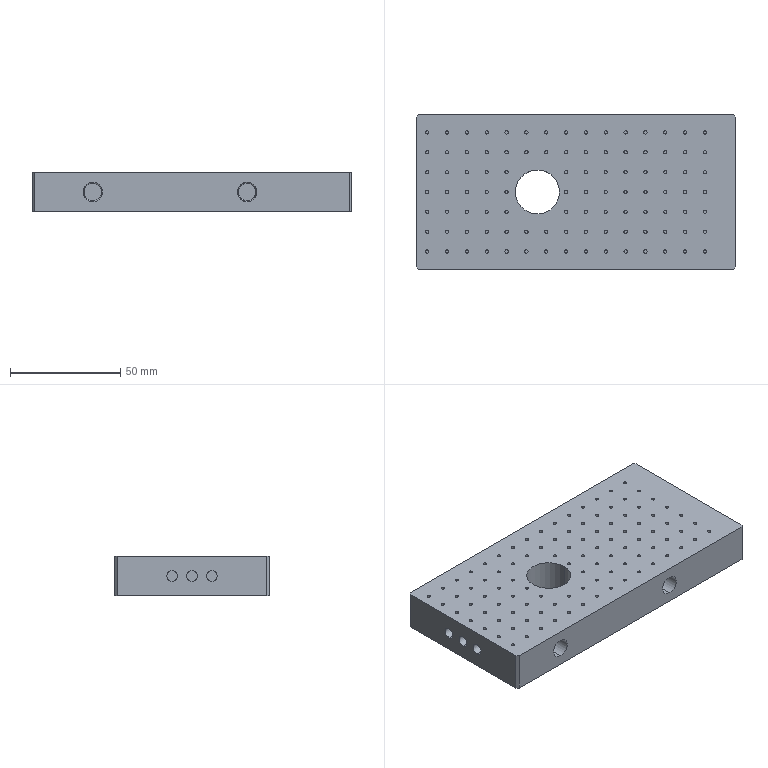Part | STEP file | 2085 Upper suction plate | 1 solid | 633 faces | box 145 x 70 x 18 mm | volume 152195 mm3 | cylinder 480 | plane 121 | cone 32 | commonest cylinder face diameters 1.5 x394 4.999 x48 5 x20 3.3 x8 8 x4 8.8 x4